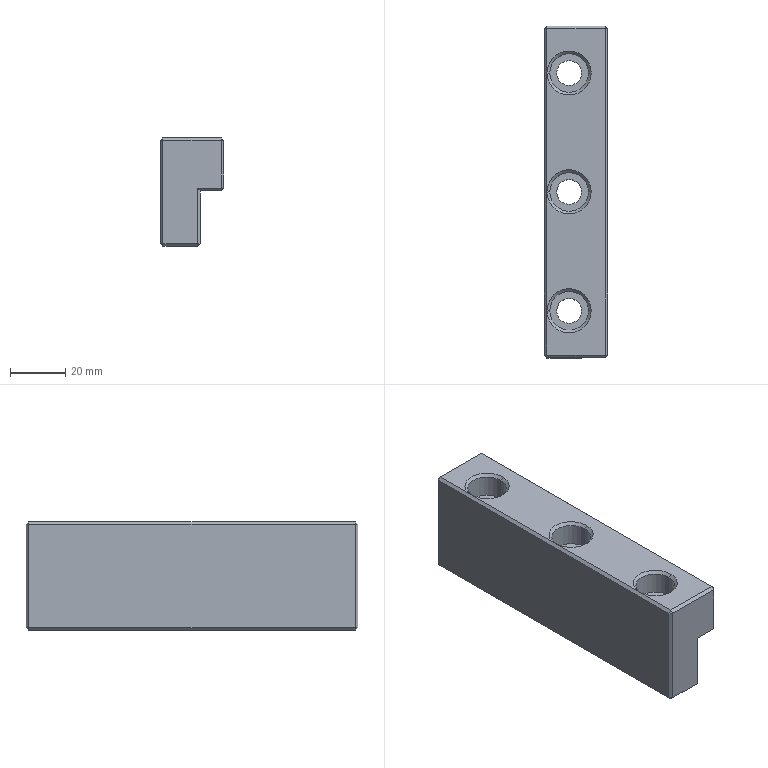Part | Creo | 1 solid | 62 faces | box 23 x 120 x 39.267 mm | volume 77513 mm3 | plane 38 | cone 12 | cylinder 12 | commonest cylinder face diameters 9 x6 14 x6